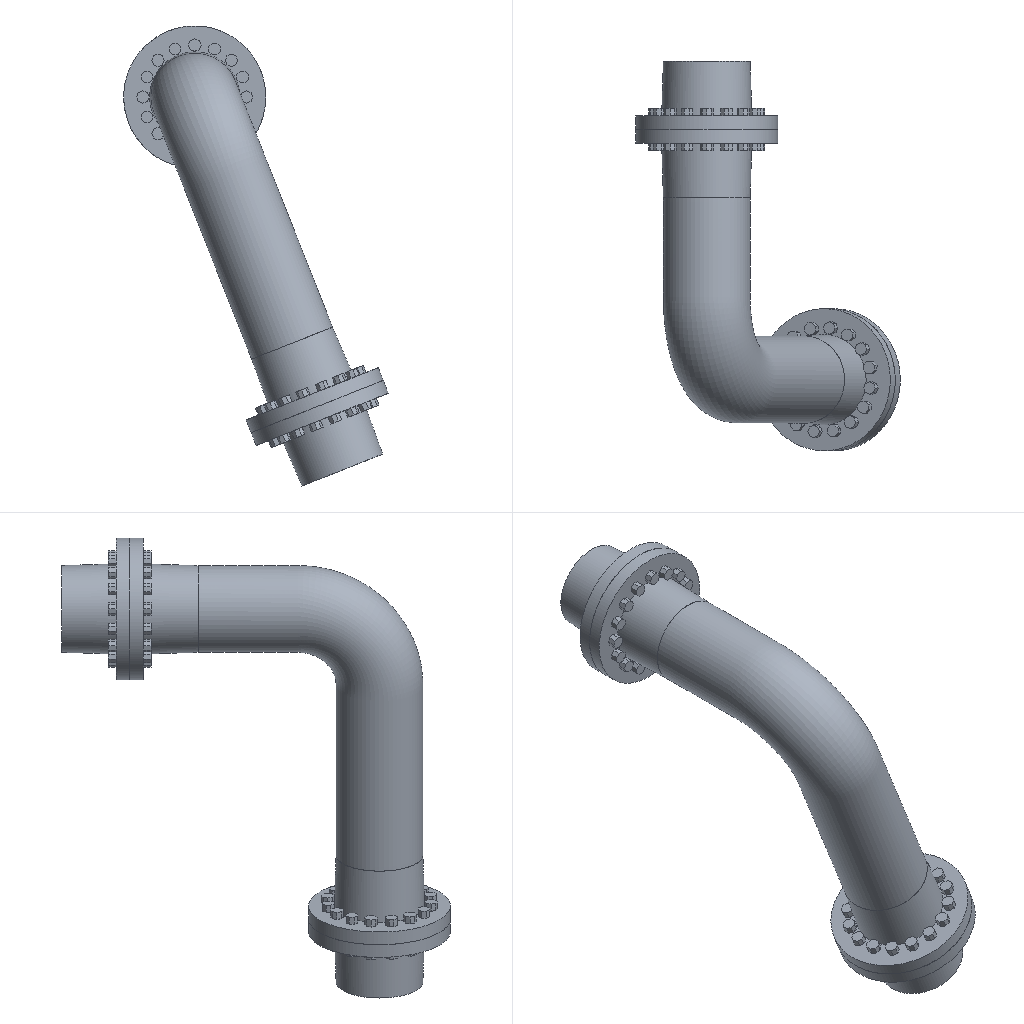Simulation study | abaqus
Set-up summary:
category,name,step,type,value,unit,region
solver,abaqus
solver,version,,,Abaqus/Explicit 2020
units,not stated in the deck,,not stated
analysis,deck,,transient,transient
load_step,Step-1,Step-1,transient
load_step,requested,,,1
mesh,nodes,,,69898
mesh,elements,,,46088
element_type,C3D8R,,solid,46088
load,load commands in deck,,count,5
bc,support commands in deck,,count,1
material,GUAN,,in results
material,SHUAN,,in results
check,setup vs results,,match,"per instance, exact: element labels, types and connectivity; labels of the nodes the elements use; coordinates of those nodes at SINGLE_PRECISION in 36 of 37 instance(s)"
Abaqus input file, long lists of numbers shortened, first 398 of 1284 lines:
*Heading
** Job name: Job-2 Model name: Model-1
** Generated by: Abaqus/CAE 2020
*Preprint, echo=NO, model=NO, history=NO, contact=NO
**
** PARTS
**
*Part, name=work-1
*Node
      1,   7.516,   71.639,    327.175
      2,   28.109,   71.639,   296.355
** (11603 more lines like these left out)
*Element, type=C3D8R
  1, 1914, 1854,  144,  143, 7833, 7773, 2131, 2140
  2, 1913, 1855, 1854, 1914, 7832, 7774, 7773, 7833
** (7830 more lines like these left out)
*Nset, nset=Set-2, generate
     1,  11605,      1
*Elset, elset=Set-2, generate
    1,  7832,     1
** Section: guan
*Solid Section, elset=Set-2, material=guan
,
*End Part
**
*Part, name=work-2
*Node
      1,   -133.467,  -53.341,   303.478
      2,   -129.716,  -53.341,   300.992
** (11398 more lines like these left out)
*Element, type=C3D8R
   1,   121,   122,   133,   162,     1,     2,    13,    42
   2,   162,   133,   134,   161,    42,    13,    14,    41
** (5638 more lines like these left out)
*Nset, nset=Set-2, generate
     1,  11400,      1
*Elset, elset=Set-2, generate
    1,  5640,     1
** Section: guan
*Solid Section, elset=Set-2, material=guan
,
*End Part
**
*Part, name=work-3
*Node
      1,   251.619,  -399.758,   -269.833
      2,   277.179,  -403.562,  -259.721
** (13338 more lines like these left out)
*Element, type=C3D8R
  1, 1985, 1926,  167,  166, 9413, 9354, 2193, 2202
  2, 1984, 1927, 1926, 1985, 9412, 9355, 9354, 9413
** (9574 more lines like these left out)
*Nset, nset=Set-2, generate
     1,  13340,      1
*Elset, elset=Set-2, generate
    1,  9576,     1
** Section: guan
*Solid Section, elset=Set-2, material=guan
,
*End Part
**
*Part, name=work-8
*Node
      1,  -77.419,   46.139,   165.583
      2,  -77.419,   46.139,   158.333
** (267 more lines like these left out)
*Element, type=C3D8R
 1, 130,  31, 123, 229,  29,   1,  30, 122
 2, 131,  32, 124, 228, 130,  31, 123, 229
** (174 more lines like these left out)
*Nset, nset=Set-1, generate
   1,  269,    1
*Elset, elset=Set-1, generate
   1,  176,    1
** Section: shuan
*Solid Section, elset=Set-1, material=shuan
,
*End Part
**
*Part, name=work-39
*Node
      1,    170.135,  -290.816,  -328.954
      2,   170.243,   -283.567,  -328.911
** (267 more lines like these left out)
*Element, type=C3D8R
 1, 130,  37, 123, 229,  29,   1,  30, 122
 2, 131,  36, 124, 228, 130,  37, 123, 229
** (174 more lines like these left out)
*Nset, nset=Set-1, generate
   1,  269,    1
*Elset, elset=Set-1, generate
   1,  176,    1
** Section: shuan
*Solid Section, elset=Set-1, material=shuan
,
*End Part
**
**
** ASSEMBLY
**
*Assembly, name=Assembly
**
*Instance, name=work-1-1, part=work-1
*End Instance
**
*Instance, name=work-2-1, part=work-2
*End Instance
**
*Instance, name=work-3-1, part=work-3
*End Instance
**
*Instance, name=work-8-1, part=work-8
   10.51,     0.5,    -0.5831
*End Instance
**
*Instance, name=work-39-1, part=work-39
   10.692,    -0.1838,     4.23
*End Instance
**
*Instance, name=work-1-2, part=work-1
 -133.819,   143.277,           0.
 -133.819,   143.277,           0.,  -133.819,   143.277,           1.,         180.
*End Instance
**
*Instance, name=work-3-2, part=work-3
156.459, -747.905, -676.855
156.459, -747.905, -676.855, 157.38, -748.043, -676.49,         180.
*End Instance
**
*Instance, name=work-39-1-rad-2, part=work-39
-124.956, -37.925, -49.433
-124.956, -37.925, -49.433, -125.324, -37.925, -48.504, 22.5
*End Instance
**
*Instance, name=work-39-1-rad-3, part=work-39
-236.848, -128.617, -93.699
-236.848, -128.617, -93.699, -237.216, -128.617, -92.769, 45.
*End Instance
**
*Instance, name=work-39-1-rad-4, part=work-39
-307.95, -258.454, -121.827
-307.95, -258.454, -121.827, -308.318, -258.454, -120.898, 67.5
*End Instance
**
*Instance, name=work-39-1-rad-5, part=work-39
-327.438, -407.67, -129.537
-327.438, -407.67, -129.537, -327.806, -407.67, -128.607, 90.
*End Instance
**
*Instance, name=work-39-1-rad-6, part=work-39
-292.343, -553.547, -115.653
-292.343, -553.547, -115.653, -292.711, -553.547, -114.723, 112.5
*End Instance
**
*Instance, name=work-39-1-rad-7, part=work-39
-208.01, -673.877, -82.29
-208.01, -673.877, -82.29, -208.378, -673.877, -81.361, 135.
*End Instance
**
*Instance, name=work-39-1-rad-8, part=work-39
-87.277, -750.341, -34.528
-87.277, -750.341, -34.528, -87.645, -750.341, -33.598, 157.5
*End Instance
**
*Instance, name=work-39-1-rad-9, part=work-39
51.475,  -771.298, 20.364
51.475,  -771.298, 20.364, 51.107,  -771.298, 21.294,         180.
*End Instance
**
*Instance, name=work-39-1-rad-10, part=work-39
187.123, -733.558, 74.027
187.123, -733.558, 74.027, 186.755, -733.558, 74.957, 202.5
*End Instance
**
*Instance, name=work-39-1-rad-11, part=work-39
299.015, -642.865, 118.293
299.015, -642.865, 118.293, 298.647, -642.865, 119.223, 225.
*End Instance
**
*Instance, name=work-39-1-rad-12, part=work-39
370.118, -513.028, 146.421
370.118, -513.028, 146.421, 370.485, -513.028, 145.491, 112.5
*End Instance
**
*Instance, name=work-39-1-rad-13, part=work-39
389.605, -363.812, 154.131
389.605, -363.812, 154.131, 389.973, -363.812, 153.201, 90.
*End Instance
**
*Instance, name=work-39-1-rad-14, part=work-39
354.511, -217.935, 140.247
354.511, -217.935, 140.247, 354.879, -217.935, 139.317, 67.5
*End Instance
**
*Instance, name=work-39-1-rad-15, part=work-39
270.178, -97.605, 106.884
270.178, -97.605, 106.884, 270.545, -97.605, 105.954, 45.
*End Instance
**
*Instance, name=work-39-1-rad-16, part=work-39
149.445, -21.141, 59.121
149.445, -21.141, 59.121, 149.812, -21.141, 58.192, 22.5
*End Instance
**
*Instance, name=work-8-1-rad-2, part=work-8
104.338,     0.5, 48.88
104.338,     0.5, 48.88, 104.338, -0.5, 48.88, 22.5
*End Instance
**
*Instance, name=work-8-1-rad-3, part=work-8
172.094,     0.5, 130.484
172.094,     0.5, 130.484, 172.094, -0.5, 130.484, 45.
*End Instance
**
*Instance, name=work-8-1-rad-4, part=work-8
203.465,     0.5, 231.805
203.465,     0.5, 231.805, 203.465, -0.5, 231.805, 67.5
*End Instance
**
*Instance, name=work-8-1-rad-5, part=work-8
  193.674,     0.5,   337.419
  193.674,     0.5,   337.419,   193.674, -0.5,   337.419, 90.
*End Instance
**
*Instance, name=work-8-1-rad-6, part=work-8
144.211,     0.5, 431.247
144.211,     0.5, 431.247, 144.211, -0.5, 431.247, 112.5
*End Instance
**
*Instance, name=work-8-1-rad-7, part=work-8
62.607,     0.5, 499.004
62.607,     0.5, 499.004, 62.607, 1.5, 499.004, 225.
*End Instance
**
*Instance, name=work-8-1-rad-8, part=work-8
-38.715,     0.5, 530.374
-38.715,     0.5, 530.374, -38.715, 1.5, 530.374, 202.5
*End Instance
**
*Instance, name=work-8-1-rad-9, part=work-8
 -144.329,     0.5,   520.583
 -144.329,     0.5,   520.583,  -144.329,     1.5,   520.583,         180.
*End Instance
**
*Instance, name=work-8-1-rad-10, part=work-8
-238.156,     0.5, 471.12
-238.156,     0.5, 471.12, -238.156, 1.5, 471.12, 157.5
*End Instance
**
*Instance, name=work-8-1-rad-11, part=work-8
-305.913,     0.5, 389.516
-305.913,     0.5, 389.516, -305.913, 1.5, 389.516, 135.
*End Instance
**
*Instance, name=work-8-1-rad-12, part=work-8
-337.284,     0.5, 288.195
-337.284,     0.5, 288.195, -337.284, 1.5, 288.195, 112.5
*End Instance
**
*Instance, name=work-8-1-rad-13, part=work-8
 -327.493,     0.5,   182.581
 -327.493,     0.5,   182.581,  -327.493, 1.5,   182.581, 90.
*End Instance
**
*Instance, name=work-8-1-rad-14, part=work-8
-278.03,     0.5, 88.753
-278.03,     0.5, 88.753, -278.03, 1.5, 88.753, 67.5
*End Instance
**
*Instance, name=work-8-1-rad-15, part=work-8
-196.426,     0.5, 20.996
-196.426,     0.5, 20.996, -196.426, 1.5, 20.996, 45.
*End Instance
**
*Instance, name=work-8-1-rad-16, part=work-8
-95.104,     0.5, -10.374
-95.104,     0.5, -10.374, -95.104, 1.5, -10.374, 22.5
*End Instance
**
*Node
      1,  -66.909,  -53.341,         260.
*Nset, nset=Set-1, instance=work-1-1, generate
     1,  11605,      1
*Nset, nset=Set-1, instance=work-2-1, generate
     1,  11400,      1
*Nset, nset=Set-1, instance=work-3-1, generate
     1,  13340,      1
*Nset, nset=Set-1, instance=work-39-1-rad-2, generate
   1,  269,    1
*Nset, nset=Set-1, instance=work-39-1-rad-10, generate
   1,  269,    1
*Nset, nset=Set-1, instance=work-39-1-rad-6, generate
   1,  269,    1
*Nset, nset=Set-1, instance=work-39-1-rad-14, generate
   1,  269,    1
*Nset, nset=Set-1, instance=work-1-2, generate
     1,  11605,      1
*Nset, nset=Set-1, instance=work-39-1-rad-4, generate
   1,  269,    1
*Nset, nset=Set-1, instance=work-39-1-rad-12, generate
   1,  269,    1
*Nset, nset=Set-1, instance=work-39-1-rad-8, generate
   1,  269,    1
*Nset, nset=Set-1, instance=work-39-1-rad-16, generate
   1,  269,    1
*Nset, nset=Set-1, instance=work-8-1, generate
   1,  269,    1
*Nset, nset=Set-1, instance=work-39-1, generate
   1,  269,    1
*Nset, nset=Set-1, instance=work-39-1-rad-3, generate
   1,  269,    1
*Nset, nset=Set-1, instance=work-39-1-rad-11, generate
   1,  269,    1
*Nset, nset=Set-1, instance=work-3-2, generate
     1,  13340,      1
*Nset, nset=Set-1, instance=work-39-1-rad-7, generate
   1,  269,    1
*Nset, nset=Set-1, instance=work-39-1-rad-15, generate
   1,  269,    1
*Nset, nset=Set-1, instance=work-39-1-rad-5, generate
   1,  269,    1
*Nset, nset=Set-1, instance=work-39-1-rad-13, generate
   1,  269,    1
*Nset, nset=Set-1, instance=work-39-1-rad-9, generate
   1,  269,    1
*Nset, nset=Set-1, instance=work-8-1-rad-2, generate
   1,  269,    1
*Nset, nset=Set-1, instance=work-8-1-rad-4, generate
   1,  269,    1
*Nset, nset=Set-1, instance=work-8-1-rad-6, generate
   1,  269,    1
*Nset, nset=Set-1, instance=work-8-1-rad-10, generate
   1,  269,    1
*Nset, nset=Set-1, instance=work-8-1-rad-14, generate
   1,  269,    1
*Nset, nset=Set-1, instance=work-8-1-rad-8, generate
   1,  269,    1
*Nset, nset=Set-1, instance=work-8-1-rad-12, generate
   1,  269,    1
*Nset, nset=Set-1, instance=work-8-1-rad-16, generate
   1,  269,    1
*Nset, nset=Set-1, instance=work-8-1-rad-3, generate
   1,  269,    1
*Nset, nset=Set-1, instance=work-8-1-rad-7, generate
   1,  269,    1
*Nset, nset=Set-1, instance=work-8-1-rad-11, generate
   1,  269,    1
*Nset, nset=Set-1, instance=work-8-1-rad-15, generate
   1,  269,    1
*Nset, nset=Set-1, instance=work-8-1-rad-5, generate
   1,  269,    1
*Nset, nset=Set-1, instance=work-8-1-rad-13, generate
   1,  269,    1
*Nset, nset=Set-1, instance=work-8-1-rad-9, generate
   1,  269,    1
*Elset, elset=Set-1, instance=work-1-1, generate
    1,  7832,     1
*Elset, elset=Set-1, instance=work-2-1, generate
    1,  5640,     1
*Elset, elset=Set-1, instance=work-3-1, generate
    1,  9576,     1
*Elset, elset=Set-1, instance=work-39-1-rad-2, generate
   1,  176,    1
*Elset, elset=Set-1, instance=work-39-1-rad-10, generate
   1,  176,    1
*Elset, elset=Set-1, instance=work-39-1-rad-6, generate
   1,  176,    1
*Elset, elset=Set-1, instance=work-39-1-rad-14, generate
   1,  176,    1
*Elset, elset=Set-1, instance=work-1-2, generate
    1,  7832,     1
*Elset, elset=Set-1, instance=work-39-1-rad-4, generate
   1,  176,    1
*Elset, elset=Set-1, instance=work-39-1-rad-12, generate
   1,  176,    1
*Elset, elset=Set-1, instance=work-39-1-rad-8, generate
   1,  176,    1
*Elset, elset=Set-1, instance=work-39-1-rad-16, generate
   1,  176,    1
*Elset, elset=Set-1, instance=work-8-1, generate
   1,  176,    1
*Elset, elset=Set-1, instance=work-39-1, generate
   1,  176,    1
*Elset, elset=Set-1, instance=work-39-1-rad-3, generate
   1,  176,    1
*Elset, elset=Set-1, instance=work-39-1-rad-11, generate
   1,  176,    1
*Elset, elset=Set-1, instance=work-3-2, generate
    1,  9576,     1
*Elset, elset=Set-1, instance=work-39-1-rad-7, generate
   1,  176,    1
*Elset, elset=Set-1, instance=work-39-1-rad-15, generate
   1,  176,    1
*Elset, elset=Set-1, instance=work-39-1-rad-5, generate
   1,  176,    1
*Elset, elset=Set-1, instance=work-39-1-rad-13, generate
   1,  176,    1
*Elset, elset=Set-1, instance=work-39-1-rad-9, generate
Last 584 lines:
*Elset, elset=_m_Surf-5_S4, internal, instance=work-3-1, generate
 7749,  9576,    21
*Surface, type=ELEMENT, name=m_Surf-5
_m_Surf-5_S4, S4
*Elset, elset=_m_Surf-7_S1, internal, instance=work-1-2
    1,    2,    3,    4,    5,    6,    7,    8,    9,   10,   11,   12,   13,   14,   15,   16
   17,   18,   19,   20,   21,   22,   23,   24,   25,   26,   27,   28,   29,   30,   31,   32
** (60 more lines like these left out)
*Surface, type=ELEMENT, name=m_Surf-7
_m_Surf-7_S1, S1
*Elset, elset=_m_Surf-9_S5, internal, instance=work-1-2, generate
 4265,  7832,    41
*Elset, elset=_m_Surf-9_S1, internal, instance=work-1-2
    1,    2,    3,    4,    5,    6,    7,    8,    9,   10,   11,   12,   13,   14,   15,   16
   17,   18,   19,   20,   21,   22,   23,   24,   25,   26,   27,   28,   29,   30,   31,   32
** (60 more lines like these left out)
*Surface, type=ELEMENT, name=m_Surf-9
_m_Surf-9_S5, S5
_m_Surf-9_S1, S1
*Elset, elset=_m_Surf-10_S3, internal, instance=work-3-2, generate
 2999,  6740,    43
*Elset, elset=_m_Surf-10_S6, internal, instance=work-3-2, generate
 7729,  9556,    21
*Elset, elset=_m_Surf-10_S1, internal, instance=work-3-2
    1,    2,    3,    4,    5,    6,    7,    8,    9,   10,   11,   12,   13,   14,   15,   16
   17,   18,   19,   20,   21,   22,   23,   24,   25,   26,   27,   28,   29,   30,   31,   32
** (60 more lines like these left out)
*Surface, type=ELEMENT, name=m_Surf-10
_m_Surf-10_S3, S3
_m_Surf-10_S6, S6
_m_Surf-10_S1, S1
*Elset, elset=_m_Surf-12_S5, internal, instance=work-1-2, generate
 4265,  7832,    41
*Elset, elset=_m_Surf-12_S1, internal, instance=work-1-2
    1,    2,    3,    4,    5,    6,    7,    8,    9,   10,   11,   12,   13,   14,   15,   16
   17,   18,   19,   20,   21,   22,   23,   24,   25,   26,   27,   28,   29,   30,   31,   32
** (60 more lines like these left out)
*Surface, type=ELEMENT, name=m_Surf-12
_m_Surf-12_S5, S5
_m_Surf-12_S1, S1
*Elset, elset=_m_Surf-13_S1, internal, instance=work-8-1
  97,  98, 107, 108, 117, 118, 130, 131, 137, 138, 147, 148, 157, 158, 167, 168
*Elset, elset=_m_Surf-13_S1, internal, instance=work-8-1-rad-2
  97,  98, 107, 108, 117, 118, 130, 131, 137, 138, 147, 148, 157, 158, 167, 168
*Elset, elset=_m_Surf-13_S1, internal, instance=work-8-1-rad-4
  97,  98, 107, 108, 117, 118, 130, 131, 137, 138, 147, 148, 157, 158, 167, 168
*Elset, elset=_m_Surf-13_S1, internal, instance=work-8-1-rad-6
  97,  98, 107, 108, 117, 118, 130, 131, 137, 138, 147, 148, 157, 158, 167, 168
*Elset, elset=_m_Surf-13_S1, internal, instance=work-8-1-rad-10
  97,  98, 107, 108, 117, 118, 130, 131, 137, 138, 147, 148, 157, 158, 167, 168
*Elset, elset=_m_Surf-13_S1, internal, instance=work-8-1-rad-14
  97,  98, 107, 108, 117, 118, 130, 131, 137, 138, 147, 148, 157, 158, 167, 168
*Elset, elset=_m_Surf-13_S1, internal, instance=work-8-1-rad-8
  97,  98, 107, 108, 117, 118, 130, 131, 137, 138, 147, 148, 157, 158, 167, 168
*Elset, elset=_m_Surf-13_S1, internal, instance=work-8-1-rad-12
  97,  98, 107, 108, 117, 118, 130, 131, 137, 138, 147, 148, 157, 158, 167, 168
*Elset, elset=_m_Surf-13_S1, internal, instance=work-8-1-rad-16
  97,  98, 107, 108, 117, 118, 130, 131, 137, 138, 147, 148, 157, 158, 167, 168
*Elset, elset=_m_Surf-13_S1, internal, instance=work-8-1-rad-3
  97,  98, 107, 108, 117, 118, 130, 131, 137, 138, 147, 148, 157, 158, 167, 168
*Elset, elset=_m_Surf-13_S1, internal, instance=work-8-1-rad-7
  97,  98, 107, 108, 117, 118, 130, 131, 137, 138, 147, 148, 157, 158, 167, 168
*Elset, elset=_m_Surf-13_S1, internal, instance=work-8-1-rad-11
  97,  98, 107, 108, 117, 118, 130, 131, 137, 138, 147, 148, 157, 158, 167, 168
*Elset, elset=_m_Surf-13_S1, internal, instance=work-8-1-rad-15
  97,  98, 107, 108, 117, 118, 130, 131, 137, 138, 147, 148, 157, 158, 167, 168
*Elset, elset=_m_Surf-13_S1, internal, instance=work-8-1-rad-5
  97,  98, 107, 108, 117, 118, 130, 131, 137, 138, 147, 148, 157, 158, 167, 168
*Elset, elset=_m_Surf-13_S1, internal, instance=work-8-1-rad-13
  97,  98, 107, 108, 117, 118, 130, 131, 137, 138, 147, 148, 157, 158, 167, 168
*Elset, elset=_m_Surf-13_S1, internal, instance=work-8-1-rad-9
  97,  98, 107, 108, 117, 118, 130, 131, 137, 138, 147, 148, 157, 158, 167, 168
*Elset, elset=_m_Surf-13_S3, internal, instance=work-8-1
  5,  6,  7,  8, 17, 18, 19, 20, 25, 26, 27, 28, 49, 50, 51, 52
 73, 74, 75, 76, 89, 90, 91, 92, 93, 94, 95, 96
*Elset, elset=_m_Surf-13_S3, internal, instance=work-8-1-rad-2
  5,  6,  7,  8, 17, 18, 19, 20, 25, 26, 27, 28, 49, 50, 51, 52
 73, 74, 75, 76, 89, 90, 91, 92, 93, 94, 95, 96
*Elset, elset=_m_Surf-13_S3, internal, instance=work-8-1-rad-4
  5,  6,  7,  8, 17, 18, 19, 20, 25, 26, 27, 28, 49, 50, 51, 52
 73, 74, 75, 76, 89, 90, 91, 92, 93, 94, 95, 96
*Elset, elset=_m_Surf-13_S3, internal, instance=work-8-1-rad-6
  5,  6,  7,  8, 17, 18, 19, 20, 25, 26, 27, 28, 49, 50, 51, 52
 73, 74, 75, 76, 89, 90, 91, 92, 93, 94, 95, 96
*Elset, elset=_m_Surf-13_S3, internal, instance=work-8-1-rad-10
  5,  6,  7,  8, 17, 18, 19, 20, 25, 26, 27, 28, 49, 50, 51, 52
 73, 74, 75, 76, 89, 90, 91, 92, 93, 94, 95, 96
*Elset, elset=_m_Surf-13_S3, internal, instance=work-8-1-rad-14
  5,  6,  7,  8, 17, 18, 19, 20, 25, 26, 27, 28, 49, 50, 51, 52
 73, 74, 75, 76, 89, 90, 91, 92, 93, 94, 95, 96
*Elset, elset=_m_Surf-13_S3, internal, instance=work-8-1-rad-8
  5,  6,  7,  8, 17, 18, 19, 20, 25, 26, 27, 28, 49, 50, 51, 52
 73, 74, 75, 76, 89, 90, 91, 92, 93, 94, 95, 96
*Elset, elset=_m_Surf-13_S3, internal, instance=work-8-1-rad-12
  5,  6,  7,  8, 17, 18, 19, 20, 25, 26, 27, 28, 49, 50, 51, 52
 73, 74, 75, 76, 89, 90, 91, 92, 93, 94, 95, 96
*Elset, elset=_m_Surf-13_S3, internal, instance=work-8-1-rad-16
  5,  6,  7,  8, 17, 18, 19, 20, 25, 26, 27, 28, 49, 50, 51, 52
 73, 74, 75, 76, 89, 90, 91, 92, 93, 94, 95, 96
*Elset, elset=_m_Surf-13_S3, internal, instance=work-8-1-rad-3
  5,  6,  7,  8, 17, 18, 19, 20, 25, 26, 27, 28, 49, 50, 51, 52
 73, 74, 75, 76, 89, 90, 91, 92, 93, 94, 95, 96
*Elset, elset=_m_Surf-13_S3, internal, instance=work-8-1-rad-7
  5,  6,  7,  8, 17, 18, 19, 20, 25, 26, 27, 28, 49, 50, 51, 52
 73, 74, 75, 76, 89, 90, 91, 92, 93, 94, 95, 96
*Elset, elset=_m_Surf-13_S3, internal, instance=work-8-1-rad-11
  5,  6,  7,  8, 17, 18, 19, 20, 25, 26, 27, 28, 49, 50, 51, 52
 73, 74, 75, 76, 89, 90, 91, 92, 93, 94, 95, 96
*Elset, elset=_m_Surf-13_S3, internal, instance=work-8-1-rad-15
  5,  6,  7,  8, 17, 18, 19, 20, 25, 26, 27, 28, 49, 50, 51, 52
 73, 74, 75, 76, 89, 90, 91, 92, 93, 94, 95, 96
*Elset, elset=_m_Surf-13_S3, internal, instance=work-8-1-rad-5
  5,  6,  7,  8, 17, 18, 19, 20, 25, 26, 27, 28, 49, 50, 51, 52
 73, 74, 75, 76, 89, 90, 91, 92, 93, 94, 95, 96
*Elset, elset=_m_Surf-13_S3, internal, instance=work-8-1-rad-13
  5,  6,  7,  8, 17, 18, 19, 20, 25, 26, 27, 28, 49, 50, 51, 52
 73, 74, 75, 76, 89, 90, 91, 92, 93, 94, 95, 96
*Elset, elset=_m_Surf-13_S3, internal, instance=work-8-1-rad-9
  5,  6,  7,  8, 17, 18, 19, 20, 25, 26, 27, 28, 49, 50, 51, 52
 73, 74, 75, 76, 89, 90, 91, 92, 93, 94, 95, 96
*Elset, elset=_m_Surf-13_S4, internal, instance=work-8-1
  9, 10, 11, 12, 21, 22, 23, 24, 29, 30, 31, 32, 53, 54, 55, 56
 81, 82, 83, 84
*Elset, elset=_m_Surf-13_S4, internal, instance=work-8-1-rad-2
  9, 10, 11, 12, 21, 22, 23, 24, 29, 30, 31, 32, 53, 54, 55, 56
 81, 82, 83, 84
*Elset, elset=_m_Surf-13_S4, internal, instance=work-8-1-rad-4
  9, 10, 11, 12, 21, 22, 23, 24, 29, 30, 31, 32, 53, 54, 55, 56
 81, 82, 83, 84
*Elset, elset=_m_Surf-13_S4, internal, instance=work-8-1-rad-6
  9, 10, 11, 12, 21, 22, 23, 24, 29, 30, 31, 32, 53, 54, 55, 56
 81, 82, 83, 84
*Elset, elset=_m_Surf-13_S4, internal, instance=work-8-1-rad-10
  9, 10, 11, 12, 21, 22, 23, 24, 29, 30, 31, 32, 53, 54, 55, 56
 81, 82, 83, 84
*Elset, elset=_m_Surf-13_S4, internal, instance=work-8-1-rad-14
  9, 10, 11, 12, 21, 22, 23, 24, 29, 30, 31, 32, 53, 54, 55, 56
 81, 82, 83, 84
*Elset, elset=_m_Surf-13_S4, internal, instance=work-8-1-rad-8
  9, 10, 11, 12, 21, 22, 23, 24, 29, 30, 31, 32, 53, 54, 55, 56
 81, 82, 83, 84
*Elset, elset=_m_Surf-13_S4, internal, instance=work-8-1-rad-12
  9, 10, 11, 12, 21, 22, 23, 24, 29, 30, 31, 32, 53, 54, 55, 56
 81, 82, 83, 84
*Elset, elset=_m_Surf-13_S4, internal, instance=work-8-1-rad-16
  9, 10, 11, 12, 21, 22, 23, 24, 29, 30, 31, 32, 53, 54, 55, 56
 81, 82, 83, 84
*Elset, elset=_m_Surf-13_S4, internal, instance=work-8-1-rad-3
  9, 10, 11, 12, 21, 22, 23, 24, 29, 30, 31, 32, 53, 54, 55, 56
 81, 82, 83, 84
*Elset, elset=_m_Surf-13_S4, internal, instance=work-8-1-rad-7
  9, 10, 11, 12, 21, 22, 23, 24, 29, 30, 31, 32, 53, 54, 55, 56
 81, 82, 83, 84
*Elset, elset=_m_Surf-13_S4, internal, instance=work-8-1-rad-11
  9, 10, 11, 12, 21, 22, 23, 24, 29, 30, 31, 32, 53, 54, 55, 56
 81, 82, 83, 84
*Elset, elset=_m_Surf-13_S4, internal, instance=work-8-1-rad-15
  9, 10, 11, 12, 21, 22, 23, 24, 29, 30, 31, 32, 53, 54, 55, 56
 81, 82, 83, 84
*Elset, elset=_m_Surf-13_S4, internal, instance=work-8-1-rad-5
  9, 10, 11, 12, 21, 22, 23, 24, 29, 30, 31, 32, 53, 54, 55, 56
 81, 82, 83, 84
*Elset, elset=_m_Surf-13_S4, internal, instance=work-8-1-rad-13
  9, 10, 11, 12, 21, 22, 23, 24, 29, 30, 31, 32, 53, 54, 55, 56
 81, 82, 83, 84
*Elset, elset=_m_Surf-13_S4, internal, instance=work-8-1-rad-9
  9, 10, 11, 12, 21, 22, 23, 24, 29, 30, 31, 32, 53, 54, 55, 56
 81, 82, 83, 84
*Elset, elset=_m_Surf-13_S2, internal, instance=work-8-1
 37, 38, 39, 40, 41, 42, 43, 44, 61, 62, 63, 64, 65, 66, 67, 68
*Elset, elset=_m_Surf-13_S2, internal, instance=work-8-1-rad-2
 37, 38, 39, 40, 41, 42, 43, 44, 61, 62, 63, 64, 65, 66, 67, 68
*Elset, elset=_m_Surf-13_S2, internal, instance=work-8-1-rad-4
 37, 38, 39, 40, 41, 42, 43, 44, 61, 62, 63, 64, 65, 66, 67, 68
*Elset, elset=_m_Surf-13_S2, internal, instance=work-8-1-rad-6
 37, 38, 39, 40, 41, 42, 43, 44, 61, 62, 63, 64, 65, 66, 67, 68
*Elset, elset=_m_Surf-13_S2, internal, instance=work-8-1-rad-10
 37, 38, 39, 40, 41, 42, 43, 44, 61, 62, 63, 64, 65, 66, 67, 68
*Elset, elset=_m_Surf-13_S2, internal, instance=work-8-1-rad-14
 37, 38, 39, 40, 41, 42, 43, 44, 61, 62, 63, 64, 65, 66, 67, 68
*Elset, elset=_m_Surf-13_S2, internal, instance=work-8-1-rad-8
 37, 38, 39, 40, 41, 42, 43, 44, 61, 62, 63, 64, 65, 66, 67, 68
*Elset, elset=_m_Surf-13_S2, internal, instance=work-8-1-rad-12
 37, 38, 39, 40, 41, 42, 43, 44, 61, 62, 63, 64, 65, 66, 67, 68
*Elset, elset=_m_Surf-13_S2, internal, instance=work-8-1-rad-16
 37, 38, 39, 40, 41, 42, 43, 44, 61, 62, 63, 64, 65, 66, 67, 68
*Elset, elset=_m_Surf-13_S2, internal, instance=work-8-1-rad-3
 37, 38, 39, 40, 41, 42, 43, 44, 61, 62, 63, 64, 65, 66, 67, 68
*Elset, elset=_m_Surf-13_S2, internal, instance=work-8-1-rad-7
 37, 38, 39, 40, 41, 42, 43, 44, 61, 62, 63, 64, 65, 66, 67, 68
*Elset, elset=_m_Surf-13_S2, internal, instance=work-8-1-rad-11
 37, 38, 39, 40, 41, 42, 43, 44, 61, 62, 63, 64, 65, 66, 67, 68
*Elset, elset=_m_Surf-13_S2, internal, instance=work-8-1-rad-15
 37, 38, 39, 40, 41, 42, 43, 44, 61, 62, 63, 64, 65, 66, 67, 68
*Elset, elset=_m_Surf-13_S2, internal, instance=work-8-1-rad-5
 37, 38, 39, 40, 41, 42, 43, 44, 61, 62, 63, 64, 65, 66, 67, 68
*Elset, elset=_m_Surf-13_S2, internal, instance=work-8-1-rad-13
 37, 38, 39, 40, 41, 42, 43, 44, 61, 62, 63, 64, 65, 66, 67, 68
*Elset, elset=_m_Surf-13_S2, internal, instance=work-8-1-rad-9
 37, 38, 39, 40, 41, 42, 43, 44, 61, 62, 63, 64, 65, 66, 67, 68
*Surface, type=ELEMENT, name=m_Surf-13
_m_Surf-13_S1, S1
_m_Surf-13_S3, S3
_m_Surf-13_S4, S4
_m_Surf-13_S2, S2
*Elset, elset=_m_Surf-15_S1, internal, instance=work-39-1
  97,  98, 107, 108, 117, 118, 127, 128, 140, 141, 147, 148, 160, 161, 167, 168
*Elset, elset=_m_Surf-15_S1, internal, instance=work-39-1-rad-2
  97,  98, 107, 108, 117, 118, 127, 128, 140, 141, 147, 148, 160, 161, 167, 168
*Elset, elset=_m_Surf-15_S1, internal, instance=work-39-1-rad-4
  97,  98, 107, 108, 117, 118, 127, 128, 140, 141, 147, 148, 160, 161, 167, 168
*Elset, elset=_m_Surf-15_S1, internal, instance=work-39-1-rad-6
  97,  98, 107, 108, 117, 118, 127, 128, 140, 141, 147, 148, 160, 161, 167, 168
*Elset, elset=_m_Surf-15_S1, internal, instance=work-39-1-rad-10
  97,  98, 107, 108, 117, 118, 127, 128, 140, 141, 147, 148, 160, 161, 167, 168
*Elset, elset=_m_Surf-15_S1, internal, instance=work-39-1-rad-14
  97,  98, 107, 108, 117, 118, 127, 128, 140, 141, 147, 148, 160, 161, 167, 168
*Elset, elset=_m_Surf-15_S1, internal, instance=work-39-1-rad-8
  97,  98, 107, 108, 117, 118, 127, 128, 140, 141, 147, 148, 160, 161, 167, 168
*Elset, elset=_m_Surf-15_S1, internal, instance=work-39-1-rad-12
  97,  98, 107, 108, 117, 118, 127, 128, 140, 141, 147, 148, 160, 161, 167, 168
*Elset, elset=_m_Surf-15_S1, internal, instance=work-39-1-rad-16
  97,  98, 107, 108, 117, 118, 127, 128, 140, 141, 147, 148, 160, 161, 167, 168
*Elset, elset=_m_Surf-15_S1, internal, instance=work-39-1-rad-3
  97,  98, 107, 108, 117, 118, 127, 128, 140, 141, 147, 148, 160, 161, 167, 168
*Elset, elset=_m_Surf-15_S1, internal, instance=work-39-1-rad-7
  97,  98, 107, 108, 117, 118, 127, 128, 140, 141, 147, 148, 160, 161, 167, 168
*Elset, elset=_m_Surf-15_S1, internal, instance=work-39-1-rad-11
  97,  98, 107, 108, 117, 118, 127, 128, 140, 141, 147, 148, 160, 161, 167, 168
*Elset, elset=_m_Surf-15_S1, internal, instance=work-39-1-rad-15
  97,  98, 107, 108, 117, 118, 127, 128, 140, 141, 147, 148, 160, 161, 167, 168
*Elset, elset=_m_Surf-15_S1, internal, instance=work-39-1-rad-5
  97,  98, 107, 108, 117, 118, 127, 128, 140, 141, 147, 148, 160, 161, 167, 168
*Elset, elset=_m_Surf-15_S1, internal, instance=work-39-1-rad-13
  97,  98, 107, 108, 117, 118, 127, 128, 140, 141, 147, 148, 160, 161, 167, 168
*Elset, elset=_m_Surf-15_S1, internal, instance=work-39-1-rad-9
  97,  98, 107, 108, 117, 118, 127, 128, 140, 141, 147, 148, 160, 161, 167, 168
*Elset, elset=_m_Surf-15_S3, internal, instance=work-39-1
  5,  6,  7,  8, 17, 18, 19, 20, 25, 26, 27, 28, 49, 50, 51, 52
 77, 78, 79, 80, 89, 90, 91, 92, 93, 94, 95, 96
*Elset, elset=_m_Surf-15_S3, internal, instance=work-39-1-rad-2
  5,  6,  7,  8, 17, 18, 19, 20, 25, 26, 27, 28, 49, 50, 51, 52
 77, 78, 79, 80, 89, 90, 91, 92, 93, 94, 95, 96
*Elset, elset=_m_Surf-15_S3, internal, instance=work-39-1-rad-4
  5,  6,  7,  8, 17, 18, 19, 20, 25, 26, 27, 28, 49, 50, 51, 52
 77, 78, 79, 80, 89, 90, 91, 92, 93, 94, 95, 96
*Elset, elset=_m_Surf-15_S3, internal, instance=work-39-1-rad-6
  5,  6,  7,  8, 17, 18, 19, 20, 25, 26, 27, 28, 49, 50, 51, 52
 77, 78, 79, 80, 89, 90, 91, 92, 93, 94, 95, 96
*Elset, elset=_m_Surf-15_S3, internal, instance=work-39-1-rad-10
  5,  6,  7,  8, 17, 18, 19, 20, 25, 26, 27, 28, 49, 50, 51, 52
 77, 78, 79, 80, 89, 90, 91, 92, 93, 94, 95, 96
*Elset, elset=_m_Surf-15_S3, internal, instance=work-39-1-rad-14
  5,  6,  7,  8, 17, 18, 19, 20, 25, 26, 27, 28, 49, 50, 51, 52
 77, 78, 79, 80, 89, 90, 91, 92, 93, 94, 95, 96
*Elset, elset=_m_Surf-15_S3, internal, instance=work-39-1-rad-8
  5,  6,  7,  8, 17, 18, 19, 20, 25, 26, 27, 28, 49, 50, 51, 52
 77, 78, 79, 80, 89, 90, 91, 92, 93, 94, 95, 96
*Elset, elset=_m_Surf-15_S3, internal, instance=work-39-1-rad-12
  5,  6,  7,  8, 17, 18, 19, 20, 25, 26, 27, 28, 49, 50, 51, 52
 77, 78, 79, 80, 89, 90, 91, 92, 93, 94, 95, 96
*Elset, elset=_m_Surf-15_S3, internal, instance=work-39-1-rad-16
  5,  6,  7,  8, 17, 18, 19, 20, 25, 26, 27, 28, 49, 50, 51, 52
 77, 78, 79, 80, 89, 90, 91, 92, 93, 94, 95, 96
*Elset, elset=_m_Surf-15_S3, internal, instance=work-39-1-rad-3
  5,  6,  7,  8, 17, 18, 19, 20, 25, 26, 27, 28, 49, 50, 51, 52
 77, 78, 79, 80, 89, 90, 91, 92, 93, 94, 95, 96
*Elset, elset=_m_Surf-15_S3, internal, instance=work-39-1-rad-7
  5,  6,  7,  8, 17, 18, 19, 20, 25, 26, 27, 28, 49, 50, 51, 52
 77, 78, 79, 80, 89, 90, 91, 92, 93, 94, 95, 96
*Elset, elset=_m_Surf-15_S3, internal, instance=work-39-1-rad-11
  5,  6,  7,  8, 17, 18, 19, 20, 25, 26, 27, 28, 49, 50, 51, 52
 77, 78, 79, 80, 89, 90, 91, 92, 93, 94, 95, 96
*Elset, elset=_m_Surf-15_S3, internal, instance=work-39-1-rad-15
  5,  6,  7,  8, 17, 18, 19, 20, 25, 26, 27, 28, 49, 50, 51, 52
 77, 78, 79, 80, 89, 90, 91, 92, 93, 94, 95, 96
*Elset, elset=_m_Surf-15_S3, internal, instance=work-39-1-rad-5
  5,  6,  7,  8, 17, 18, 19, 20, 25, 26, 27, 28, 49, 50, 51, 52
 77, 78, 79, 80, 89, 90, 91, 92, 93, 94, 95, 96
*Elset, elset=_m_Surf-15_S3, internal, instance=work-39-1-rad-13
  5,  6,  7,  8, 17, 18, 19, 20, 25, 26, 27, 28, 49, 50, 51, 52
 77, 78, 79, 80, 89, 90, 91, 92, 93, 94, 95, 96
*Elset, elset=_m_Surf-15_S3, internal, instance=work-39-1-rad-9
  5,  6,  7,  8, 17, 18, 19, 20, 25, 26, 27, 28, 49, 50, 51, 52
 77, 78, 79, 80, 89, 90, 91, 92, 93, 94, 95, 96
*Elset, elset=_m_Surf-15_S4, internal, instance=work-39-1
  9, 10, 11, 12, 21, 22, 23, 24, 29, 30, 31, 32, 53, 54, 55, 56
 81, 82, 83, 84
*Elset, elset=_m_Surf-15_S4, internal, instance=work-39-1-rad-2
  9, 10, 11, 12, 21, 22, 23, 24, 29, 30, 31, 32, 53, 54, 55, 56
 81, 82, 83, 84
*Elset, elset=_m_Surf-15_S4, internal, instance=work-39-1-rad-4
  9, 10, 11, 12, 21, 22, 23, 24, 29, 30, 31, 32, 53, 54, 55, 56
 81, 82, 83, 84
*Elset, elset=_m_Surf-15_S4, internal, instance=work-39-1-rad-6
  9, 10, 11, 12, 21, 22, 23, 24, 29, 30, 31, 32, 53, 54, 55, 56
 81, 82, 83, 84
*Elset, elset=_m_Surf-15_S4, internal, instance=work-39-1-rad-10
  9, 10, 11, 12, 21, 22, 23, 24, 29, 30, 31, 32, 53, 54, 55, 56
 81, 82, 83, 84
*Elset, elset=_m_Surf-15_S4, internal, instance=work-39-1-rad-14
  9, 10, 11, 12, 21, 22, 23, 24, 29, 30, 31, 32, 53, 54, 55, 56
 81, 82, 83, 84
*Elset, elset=_m_Surf-15_S4, internal, instance=work-39-1-rad-8
  9, 10, 11, 12, 21, 22, 23, 24, 29, 30, 31, 32, 53, 54, 55, 56
 81, 82, 83, 84
*Elset, elset=_m_Surf-15_S4, internal, instance=work-39-1-rad-12
  9, 10, 11, 12, 21, 22, 23, 24, 29, 30, 31, 32, 53, 54, 55, 56
 81, 82, 83, 84
*Elset, elset=_m_Surf-15_S4, internal, instance=work-39-1-rad-16
  9, 10, 11, 12, 21, 22, 23, 24, 29, 30, 31, 32, 53, 54, 55, 56
 81, 82, 83, 84
*Elset, elset=_m_Surf-15_S4, internal, instance=work-39-1-rad-3
  9, 10, 11, 12, 21, 22, 23, 24, 29, 30, 31, 32, 53, 54, 55, 56
 81, 82, 83, 84
*Elset, elset=_m_Surf-15_S4, internal, instance=work-39-1-rad-7
  9, 10, 11, 12, 21, 22, 23, 24, 29, 30, 31, 32, 53, 54, 55, 56
 81, 82, 83, 84
*Elset, elset=_m_Surf-15_S4, internal, instance=work-39-1-rad-11
  9, 10, 11, 12, 21, 22, 23, 24, 29, 30, 31, 32, 53, 54, 55, 56
 81, 82, 83, 84
*Elset, elset=_m_Surf-15_S4, internal, instance=work-39-1-rad-15
  9, 10, 11, 12, 21, 22, 23, 24, 29, 30, 31, 32, 53, 54, 55, 56
 81, 82, 83, 84
*Elset, elset=_m_Surf-15_S4, internal, instance=work-39-1-rad-5
  9, 10, 11, 12, 21, 22, 23, 24, 29, 30, 31, 32, 53, 54, 55, 56
 81, 82, 83, 84
*Elset, elset=_m_Surf-15_S4, internal, instance=work-39-1-rad-13
  9, 10, 11, 12, 21, 22, 23, 24, 29, 30, 31, 32, 53, 54, 55, 56
 81, 82, 83, 84
*Elset, elset=_m_Surf-15_S4, internal, instance=work-39-1-rad-9
  9, 10, 11, 12, 21, 22, 23, 24, 29, 30, 31, 32, 53, 54, 55, 56
 81, 82, 83, 84
*Elset, elset=_m_Surf-15_S2, internal, instance=work-39-1
 37, 38, 39, 40, 41, 42, 43, 44, 61, 62, 63, 64, 65, 66, 67, 68
*Elset, elset=_m_Surf-15_S2, internal, instance=work-39-1-rad-2
 37, 38, 39, 40, 41, 42, 43, 44, 61, 62, 63, 64, 65, 66, 67, 68
*Elset, elset=_m_Surf-15_S2, internal, instance=work-39-1-rad-4
 37, 38, 39, 40, 41, 42, 43, 44, 61, 62, 63, 64, 65, 66, 67, 68
*Elset, elset=_m_Surf-15_S2, internal, instance=work-39-1-rad-6
 37, 38, 39, 40, 41, 42, 43, 44, 61, 62, 63, 64, 65, 66, 67, 68
*Elset, elset=_m_Surf-15_S2, internal, instance=work-39-1-rad-10
 37, 38, 39, 40, 41, 42, 43, 44, 61, 62, 63, 64, 65, 66, 67, 68
*Elset, elset=_m_Surf-15_S2, internal, instance=work-39-1-rad-14
 37, 38, 39, 40, 41, 42, 43, 44, 61, 62, 63, 64, 65, 66, 67, 68
*Elset, elset=_m_Surf-15_S2, internal, instance=work-39-1-rad-8
 37, 38, 39, 40, 41, 42, 43, 44, 61, 62, 63, 64, 65, 66, 67, 68
*Elset, elset=_m_Surf-15_S2, internal, instance=work-39-1-rad-12
 37, 38, 39, 40, 41, 42, 43, 44, 61, 62, 63, 64, 65, 66, 67, 68
*Elset, elset=_m_Surf-15_S2, internal, instance=work-39-1-rad-16
 37, 38, 39, 40, 41, 42, 43, 44, 61, 62, 63, 64, 65, 66, 67, 68
*Elset, elset=_m_Surf-15_S2, internal, instance=work-39-1-rad-3
 37, 38, 39, 40, 41, 42, 43, 44, 61, 62, 63, 64, 65, 66, 67, 68
*Elset, elset=_m_Surf-15_S2, internal, instance=work-39-1-rad-7
 37, 38, 39, 40, 41, 42, 43, 44, 61, 62, 63, 64, 65, 66, 67, 68
*Elset, elset=_m_Surf-15_S2, internal, instance=work-39-1-rad-11
 37, 38, 39, 40, 41, 42, 43, 44, 61, 62, 63, 64, 65, 66, 67, 68
*Elset, elset=_m_Surf-15_S2, internal, instance=work-39-1-rad-15
 37, 38, 39, 40, 41, 42, 43, 44, 61, 62, 63, 64, 65, 66, 67, 68
*Elset, elset=_m_Surf-15_S2, internal, instance=work-39-1-rad-5
 37, 38, 39, 40, 41, 42, 43, 44, 61, 62, 63, 64, 65, 66, 67, 68
*Elset, elset=_m_Surf-15_S2, internal, instance=work-39-1-rad-13
 37, 38, 39, 40, 41, 42, 43, 44, 61, 62, 63, 64, 65, 66, 67, 68
*Elset, elset=_m_Surf-15_S2, internal, instance=work-39-1-rad-9
 37, 38, 39, 40, 41, 42, 43, 44, 61, 62, 63, 64, 65, 66, 67, 68
*Surface, type=ELEMENT, name=m_Surf-15
_m_Surf-15_S1, S1
_m_Surf-15_S3, S3
_m_Surf-15_S4, S4
_m_Surf-15_S2, S2
*Elset, elset=_s_Surf-5_S1, internal, instance=work-2-1, generate
 5581,  5640,     1
*Surface, type=ELEMENT, name=s_Surf-5
_s_Surf-5_S1, S1
*Elset, elset=_s_Surf-7_S5, internal, instance=work-1-1, generate
 4265,  7832,    41
*Elset, elset=_s_Surf-7_S1, internal, instance=work-1-1
    1,    2,    3,    4,    5,    6,    7,    8,    9,   10,   11,   12,   13,   14,   15,   16
   17,   18,   19,   20,   21,   22,   23,   24,   25,   26,   27,   28,   29,   30,   31,   32
** (60 more lines like these left out)
*Surface, type=ELEMENT, name=s_Surf-7
_s_Surf-7_S5, S5
_s_Surf-7_S1, S1
*Elset, elset=_s_Surf-10_S3, internal, instance=work-3-1, generate
 2999,  6740,    43
*Elset, elset=_s_Surf-10_S6, internal, instance=work-3-1, generate
 7729,  9556,    21
*Elset, elset=_s_Surf-10_S1, internal, instance=work-3-1
    1,    2,    3,    4,    5,    6,    7,    8,    9,   10,   11,   12,   13,   14,   15,   16
   17,   18,   19,   20,   21,   22,   23,   24,   25,   26,   27,   28,   29,   30,   31,   32
** (60 more lines like these left out)
*Surface, type=ELEMENT, name=s_Surf-10
_s_Surf-10_S3, S3
_s_Surf-10_S6, S6
_s_Surf-10_S1, S1
*Elset, elset=_s_Surf-13_S4, internal, instance=work-1-1
    7,   47,   48,   49,   50,   58,   62,   85,   86,   87,  101,  102,  110,  112,  125,  146
  171,  172,  176,  186,  199,  203,  209,  216,  239,  243,  253,  293,  294,  295,  296,  304
** (22 more lines like these left out)
*Elset, elset=_s_Surf-13_S4, internal, instance=work-1-2
    7,   47,   48,   49,   50,   58,   62,   85,   86,   87,  101,  102,  110,  112,  125,  146
  171,  172,  176,  186,  199,  203,  209,  216,  239,  243,  253,  293,  294,  295,  296,  304
** (22 more lines like these left out)
*Elset, elset=_s_Surf-13_S5, internal, instance=work-1-1
   51,   52,   63,   88,  103,  147,  173,  177,  187,  200,  204,  217,  218,  219,  235,  244
  297,  298,  309,  334,  349,  393,  419,  423,  433,  446,  450,  463,  464,  465,  481,  490
** (17 more lines like these left out)
*Elset, elset=_s_Surf-13_S5, internal, instance=work-1-2
   51,   52,   63,   88,  103,  147,  173,  177,  187,  200,  204,  217,  218,  219,  235,  244
  297,  298,  309,  334,  349,  393,  419,  423,  433,  446,  450,  463,  464,  465,  481,  490
** (17 more lines like these left out)
*Elset, elset=_s_Surf-13_S6, internal, instance=work-1-1
    8,   10,   12,  126,  127,  128,  245,  254,  256,  258,  372,  373,  374,  491,  500,  502
  504,  618,  619,  620,  737,  746,  748,  750,  864,  865,  866,  983, 1096, 1166, 1342, 1412
** (3 more lines like these left out)
*Elset, elset=_s_Surf-13_S6, internal, instance=work-1-2
    8,   10,   12,  126,  127,  128,  245,  254,  256,  258,  372,  373,  374,  491,  500,  502
  504,  618,  619,  620,  737,  746,  748,  750,  864,  865,  866,  983, 1096, 1166, 1342, 1412
** (3 more lines like these left out)
*Elset, elset=_s_Surf-13_S3, internal, instance=work-1-1
 2108, 2109, 2110, 2111, 2169, 2170, 2171, 2356, 2357, 2358, 2359, 2417, 2418, 2419, 2604, 2605
 2606, 2607, 2665, 2666, 2667, 2852, 2853, 2854, 2855, 2913, 2914, 2915
*Elset, elset=_s_Surf-13_S3, internal, instance=work-1-2
 2108, 2109, 2110, 2111, 2169, 2170, 2171, 2356, 2357, 2358, 2359, 2417, 2418, 2419, 2604, 2605
 2606, 2607, 2665, 2666, 2667, 2852, 2853, 2854, 2855, 2913, 2914, 2915
*Surface, type=ELEMENT, name=s_Surf-13
_s_Surf-13_S4, S4
_s_Surf-13_S5, S5
_s_Surf-13_S6, S6
_s_Surf-13_S3, S3
*Elset, elset=_s_Surf-15_S4, internal, instance=work-3-1
    7,   43,   48,   56,   77,  104,  105,  108,  120,  147,  173,  174,  175,  180,  196,  205
  229,  230,  231,  241,  246,  253,  289,  294,  302,  323,  350,  351,  354,  366,  393,  419
** (21 more lines like these left out)
*Elset, elset=_s_Surf-15_S4, internal, instance=work-3-2
    7,   43,   48,   56,   77,  104,  105,  108,  120,  147,  173,  174,  175,  180,  196,  205
  229,  230,  231,  241,  246,  253,  289,  294,  302,  323,  350,  351,  354,  366,  393,  419
** (21 more lines like these left out)
*Elset, elset=_s_Surf-15_S5, internal, instance=work-3-1
    8,    9,   10,   44,   49,   57,   58,   59,   78,  106,  109,  121,  122,  123,  124,  148
  176,  181,  197,  206,  232,  235,  242,  254,  255,  256,  290,  295,  303,  304,  305,  324
** (18 more lines like these left out)
*Elset, elset=_s_Surf-15_S5, internal, instance=work-3-2
    8,    9,   10,   44,   49,   57,   58,   59,   78,  106,  109,  121,  122,  123,  124,  148
  176,  181,  197,  206,  232,  235,  242,  254,  255,  256,  290,  295,  303,  304,  305,  324
** (18 more lines like these left out)
*Elset, elset=_s_Surf-15_S6, internal, instance=work-3-1
  112,  182,  237,  358,  428,  483,  604,  674,  729,  850,  920,  975, 1096, 1166, 1221, 1342
 1412, 1467, 1588, 1658, 1713, 1834, 1904, 1959, 1976, 1978, 1980, 2089, 2090, 2091, 2214, 2223
** (3 more lines like these left out)
*Elset, elset=_s_Surf-15_S6, internal, instance=work-3-2
  112,  182,  237,  358,  428,  483,  604,  674,  729,  850,  920,  975, 1096, 1166, 1221, 1342
 1412, 1467, 1588, 1658, 1713, 1834, 1904, 1959, 1976, 1978, 1980, 2089, 2090, 2091, 2214, 2223
** (3 more lines like these left out)
*Surface, type=ELEMENT, name=s_Surf-15
_s_Surf-15_S4, S4
_s_Surf-15_S5, S5
_s_Surf-15_S6, S6
*Elset, elset=_s_Surf-19_S1, internal, instance=work-2-1, generate
 5581,  5640,     1
*Elset, elset=_s_Surf-19_S2, internal, instance=work-2-1, generate
  1,  60,   1
*Surface, type=ELEMENT, name=s_Surf-19
_s_Surf-19_S1, S1
_s_Surf-19_S2, S2
*Elset, elset=_s_Surf-20_S3, internal, instance=work-1-1
 4225, 4226, 4227, 4228, 4229, 4230, 4231, 4232, 4233, 4234, 4235, 4236, 4237, 4238, 4239, 4240
 4241, 4242, 4243, 4244, 4266, 4267, 4268, 4269, 4270, 4271, 4272, 4273, 4274, 4275, 4276, 4277
** (108 more lines like these left out)
*Elset, elset=_s_Surf-20_S6, internal, instance=work-1-1, generate
 4265,  7832,    41
*Surface, type=ELEMENT, name=s_Surf-20
_s_Surf-20_S3, S3
_s_Surf-20_S6, S6
** Constraint: Constraint-1
*Tie, name=Constraint-1, adjust=yes
s_Surf-19, m_Surf-5
** Constraint: Constraint-2
*Coupling, constraint name=Constraint-2, ref node=m_Set-6, surface=s_Surf-20
*Kinematic
*End Assembly
*Amplitude, name=Amp-1
             0.,              0.,            0.01,              1.
**
** MATERIALS
**
*Material, name=guan
*Conductivity
1.,
*Density
 1.5e-09,
*Elastic
30000., 0.33
*Expansion
 3e-05,
*Material, name=shuan
*Conductivity
45.,
*Density
 7.8e-09,
*Elastic
200000., 0.25
*Expansion
 1.4e-05,
**
** INTERACTION PROPERTIES
**
*Surface Interaction, name=IntProp-1
*Friction
 0.1,
*Surface Behavior, pressure-overclosure=HARD
**
** PREDEFINED FIELDS
**
** Name: Predefined Field-1   Type: Temperature
*Initial Conditions, type=TEMPERATURE
Set-1, -180.
** ----------------------------------------------------------------
**
** STEP: Step-1
**
*Step, name=Step-1, nlgeom=YES
*Dynamic, Explicit
, 0.01
*Bulk Viscosity
0.06, 1.2
** Mass Scaling: Semi-Automatic
**               Whole Model
*Fixed Mass Scaling, factor=50.
**
** BOUNDARY CONDITIONS
**
** Name: BC-1 Type: 对称/反对称/完全固定
*Boundary
Set-5, ENCASTRE
**
** LOADS
**
** Name: Load-1   Type: Pressure
*Dsload
Surf-2, P, 20.
** Name: Load-2   Type: Pressure
*Dsload
Surf-3, P, 20.
** Name: Load-3   Type: Pressure
*Dsload, amplitude=Amp-1
Surf-18, P, 4.
** Name: Load-4   Type: Moment
*Cload, amplitude=Amp-1
Set-7, 5, 45110.
**
** PREDEFINED FIELDS
**
** Name: Predefined Field-1   Type: Temperature
*Temperature
Set-1, 30.
**
** INTERACTIONS
**
** Interaction: Int-5
*Contact, op=NEW
*Contact Inclusions, ALL EXTERIOR
*Contact Property Assignment
 ,  , IntProp-1
**
** OUTPUT REQUESTS
**
*Restart, write, number interval=1, time marks=NO
**
** FIELD OUTPUT: F-Output-1
**
*Output, field, number interval=50
*Node Output
A, AR, AT, CF, RF, RM, RT, U
UR, UT, V, VR, VT
*Element Output, directions=YES
E, LE, MISES, MISESMAX, PE, PEEQ, PEMAG, S, SF
*Contact Output
CDISP, CSTRESS
**
** HISTORY OUTPUT: H-Output-1
**
*Output, history, variable=PRESELECT, frequency=1
*End Step
Results summary:
result,step,Step-1,completed,increments=37258 time=0.01/0.01
result,analysis,,,transient
result,last_loadstep,,,1
result,primary field,,,U
result,reaction total,,FX,15568.011,model units
result,reaction total,,FY,78728.113,model units
result,reaction total,,FZ,-37305.636,model units